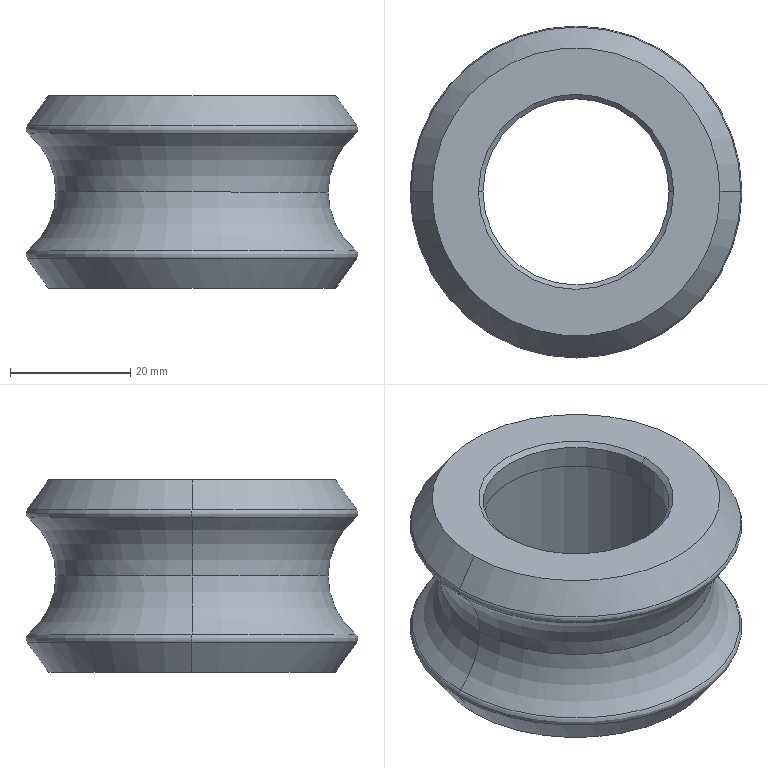Part | STEP file | ROLLER LINEAR GUIDE_01 | 1 solid | 31 faces | box 55.257 x 55.257 x 32 mm | volume 32346 mm3 | torus 10 | cylinder 8 | cone 8 | plane 5 | commonest cylinder face diameters 35 x4 31 x2 37.2 x2
STEP:
#1=CARTESIAN_POINT('',(-62.431,0.,-9.68));
#2=VERTEX_POINT('',#1);
#3=CARTESIAN_POINT('',(-57.839,0.,0.));
#4=VERTEX_POINT('',#3);
#5=CARTESIAN_POINT('',(-70.339,0.,0.));
#6=DIRECTION('',(0.,-1.,0.));
#7=DIRECTION('',(0.,0.,-1.));
#8=AXIS2_PLACEMENT_3D('',#5,#6,#7);
#9=CIRCLE('',#8,12.5);
#10=EDGE_CURVE('',#2,#4,#9,.T.);
#11=ORIENTED_EDGE('',*,*,#10,.T.);
#12=CARTESIAN_POINT('',(-12.5,0.,0.));
#13=VERTEX_POINT('',#12);
#14=CARTESIAN_POINT('',(-35.17,0.,0.));
#15=DIRECTION('',(0.,0.,-1.));
#16=DIRECTION('',(-1.,0.,0.));
#17=AXIS2_PLACEMENT_3D('',#14,#15,#16);
#18=CIRCLE('',#17,22.67);
#19=EDGE_CURVE('',#4,#13,#18,.T.);
#20=ORIENTED_EDGE('',*,*,#19,.T.);
#21=CARTESIAN_POINT('',(-7.908,0.,-9.68));
#22=VERTEX_POINT('',#21);
#23=CARTESIAN_POINT('',(0.,0.,0.));
#24=DIRECTION('',(0.,1.,0.));
#25=DIRECTION('',(-1.,0.,0.));
#26=AXIS2_PLACEMENT_3D('',#23,#24,#25);
#27=CIRCLE('',#26,12.5);
#28=EDGE_CURVE('',#22,#13,#27,.T.);
#29=ORIENTED_EDGE('',*,*,#28,.F.);
#30=CARTESIAN_POINT('',(-35.17,0.,-9.68));
#31=DIRECTION('',(0.,0.,1.));
#32=DIRECTION('',(1.,0.,0.));
#33=AXIS2_PLACEMENT_3D('',#30,#31,#32);
#34=CIRCLE('',#33,27.261);
#35=EDGE_CURVE('',#22,#2,#34,.T.);
#36=ORIENTED_EDGE('',*,*,#35,.T.);
#37=EDGE_LOOP('',(#11,#20,#29,#36));
#38=FACE_OUTER_BOUND('',#37,.T.);
#39=CARTESIAN_POINT('',(-35.17,0.,0.));
#40=DIRECTION('',(0.,0.,-1.));
#41=DIRECTION('',(-1.,0.,0.));
#42=AXIS2_PLACEMENT_3D('',#39,#40,#41);
#43=TOROIDAL_SURFACE('',#42,35.17,12.5);
#44=ADVANCED_FACE('',(#38),#43,.F.);
#45=ORIENTED_EDGE('',*,*,#28,.T.);
#46=CARTESIAN_POINT('',(-35.17,0.,0.));
#47=DIRECTION('',(0.,0.,-1.));
#48=DIRECTION('',(-1.,0.,0.));
#49=AXIS2_PLACEMENT_3D('',#46,#47,#48);
#50=CIRCLE('',#49,22.67);
#51=EDGE_CURVE('',#13,#4,#50,.T.);
#52=ORIENTED_EDGE('',*,*,#51,.T.);
#53=ORIENTED_EDGE('',*,*,#10,.F.);
#54=CARTESIAN_POINT('',(-35.17,0.,-9.68));
#55=DIRECTION('',(0.,0.,1.));
#56=DIRECTION('',(1.,0.,0.));
#57=AXIS2_PLACEMENT_3D('',#54,#55,#56);
#58=CIRCLE('',#57,27.261);
#59=EDGE_CURVE('',#2,#22,#58,.T.);
#60=ORIENTED_EDGE('',*,*,#59,.T.);
#61=EDGE_LOOP('',(#45,#52,#53,#60));
#62=FACE_OUTER_BOUND('',#61,.T.);
#63=CARTESIAN_POINT('',(-35.17,0.,0.));
#64=DIRECTION('',(0.,0.,-1.));
#65=DIRECTION('',(-1.,0.,0.));
#66=AXIS2_PLACEMENT_3D('',#63,#64,#65);
#67=TOROIDAL_SURFACE('',#66,35.17,12.5);
#68=ADVANCED_FACE('',(#62),#67,.F.);
#69=CARTESIAN_POINT('',(-16.57,0.,-11.8));
#70=VERTEX_POINT('',#69);
#71=CARTESIAN_POINT('',(-53.77,0.,-11.8));
#72=VERTEX_POINT('',#71);
#73=CARTESIAN_POINT('',(-35.17,0.,-11.8));
#74=DIRECTION('',(0.,0.,-1.));
#75=DIRECTION('',(-1.,0.,0.));
#76=AXIS2_PLACEMENT_3D('',#73,#74,#75);
#77=CIRCLE('',#76,18.6);
#78=EDGE_CURVE('',#70,#72,#77,.T.);
#79=ORIENTED_EDGE('',*,*,#78,.F.);
#80=CARTESIAN_POINT('',(-16.57,0.,-13.2));
#81=VERTEX_POINT('',#80);
#82=CARTESIAN_POINT('',(-16.57,0.,-16.));
#83=DIRECTION('',(0.,0.,-1.));
#84=VECTOR('',#83,1000.);
#85=LINE('',#82,#84);
#86=EDGE_CURVE('',#70,#81,#85,.T.);
#87=ORIENTED_EDGE('',*,*,#86,.T.);
#88=CARTESIAN_POINT('',(-53.77,0.,-13.2));
#89=VERTEX_POINT('',#88);
#90=CARTESIAN_POINT('',(-35.17,0.,-13.2));
#91=DIRECTION('',(0.,0.,-1.));
#92=DIRECTION('',(-1.,0.,0.));
#93=AXIS2_PLACEMENT_3D('',#90,#91,#92);
#94=CIRCLE('',#93,18.6);
#95=EDGE_CURVE('',#81,#89,#94,.T.);
#96=ORIENTED_EDGE('',*,*,#95,.T.);
#97=CARTESIAN_POINT('',(-53.77,0.,-16.));
#98=DIRECTION('',(0.,0.,-1.));
#99=VECTOR('',#98,1000.);
#100=LINE('',#97,#99);
#101=EDGE_CURVE('',#72,#89,#100,.T.);
#102=ORIENTED_EDGE('',*,*,#101,.F.);
#103=EDGE_LOOP('',(#79,#87,#96,#102));
#104=FACE_OUTER_BOUND('',#103,.T.);
#105=CARTESIAN_POINT('',(-35.17,0.,-16.));
#106=DIRECTION('',(0.,0.,-1.));
#107=DIRECTION('',(-1.,0.,0.));
#108=AXIS2_PLACEMENT_3D('',#105,#106,#107);
#109=CYLINDRICAL_SURFACE('',#108,18.6);
#110=ADVANCED_FACE('',(#104),#109,.F.);
#111=CARTESIAN_POINT('',(-62.431,0.,9.68));
#112=VERTEX_POINT('',#111);
#113=CARTESIAN_POINT('',(-7.908,0.,9.68));
#114=VERTEX_POINT('',#113);
#115=CARTESIAN_POINT('',(-35.17,0.,9.68));
#116=DIRECTION('',(0.,0.,-1.));
#117=DIRECTION('',(-1.,0.,0.));
#118=AXIS2_PLACEMENT_3D('',#115,#116,#117);
#119=CIRCLE('',#118,27.261);
#120=EDGE_CURVE('',#112,#114,#119,.T.);
#121=ORIENTED_EDGE('',*,*,#120,.F.);
#122=CARTESIAN_POINT('',(-62.617,0.,11.028));
#123=VERTEX_POINT('',#122);
#124=CARTESIAN_POINT('',(-61.798,0.,10.455));
#125=DIRECTION('',(0.,1.,0.));
#126=DIRECTION('',(-1.,0.,0.));
#127=AXIS2_PLACEMENT_3D('',#124,#125,#126);
#128=CIRCLE('',#127,1.);
#129=EDGE_CURVE('',#112,#123,#128,.T.);
#130=ORIENTED_EDGE('',*,*,#129,.T.);
#131=CARTESIAN_POINT('',(-7.722,0.,11.028));
#132=VERTEX_POINT('',#131);
#133=CARTESIAN_POINT('',(-35.17,0.,11.028));
#134=DIRECTION('',(0.,0.,1.));
#135=DIRECTION('',(1.,0.,0.));
#136=AXIS2_PLACEMENT_3D('',#133,#134,#135);
#137=CIRCLE('',#136,27.448);
#138=EDGE_CURVE('',#132,#123,#137,.T.);
#139=ORIENTED_EDGE('',*,*,#138,.F.);
#140=CARTESIAN_POINT('',(-8.541,0.,10.455));
#141=DIRECTION('',(0.,-1.,0.));
#142=DIRECTION('',(0.,0.,-1.));
#143=AXIS2_PLACEMENT_3D('',#140,#141,#142);
#144=CIRCLE('',#143,1.);
#145=EDGE_CURVE('',#114,#132,#144,.T.);
#146=ORIENTED_EDGE('',*,*,#145,.F.);
#147=EDGE_LOOP('',(#121,#130,#139,#146));
#148=FACE_OUTER_BOUND('',#147,.T.);
#149=CARTESIAN_POINT('',(-35.17,0.,10.455));
#150=DIRECTION('',(0.,0.,1.));
#151=DIRECTION('',(1.,0.,0.));
#152=AXIS2_PLACEMENT_3D('',#149,#150,#151);
#153=TOROIDAL_SURFACE('',#152,26.629,1.);
#154=ADVANCED_FACE('',(#148),#153,.T.);
#155=CARTESIAN_POINT('',(-62.617,0.,-11.028));
#156=VERTEX_POINT('',#155);
#157=CARTESIAN_POINT('',(-7.722,0.,-11.028));
#158=VERTEX_POINT('',#157);
#159=CARTESIAN_POINT('',(-35.17,0.,-11.028));
#160=DIRECTION('',(0.,0.,-1.));
#161=DIRECTION('',(-1.,0.,0.));
#162=AXIS2_PLACEMENT_3D('',#159,#160,#161);
#163=CIRCLE('',#162,27.448);
#164=EDGE_CURVE('',#156,#158,#163,.T.);
#165=ORIENTED_EDGE('',*,*,#164,.F.);
#166=CARTESIAN_POINT('',(-61.798,0.,-10.455));
#167=DIRECTION('',(0.,1.,0.));
#168=DIRECTION('',(-1.,0.,0.));
#169=AXIS2_PLACEMENT_3D('',#166,#167,#168);
#170=CIRCLE('',#169,1.);
#171=EDGE_CURVE('',#156,#2,#170,.T.);
#172=ORIENTED_EDGE('',*,*,#171,.T.);
#173=ORIENTED_EDGE('',*,*,#35,.F.);
#174=CARTESIAN_POINT('',(-8.541,0.,-10.455));
#175=DIRECTION('',(0.,-1.,0.));
#176=DIRECTION('',(0.,0.,-1.));
#177=AXIS2_PLACEMENT_3D('',#174,#175,#176);
#178=CIRCLE('',#177,1.);
#179=EDGE_CURVE('',#158,#22,#178,.T.);
#180=ORIENTED_EDGE('',*,*,#179,.F.);
#181=EDGE_LOOP('',(#165,#172,#173,#180));
#182=FACE_OUTER_BOUND('',#181,.T.);
#183=CARTESIAN_POINT('',(-35.17,0.,-10.455));
#184=DIRECTION('',(0.,0.,1.));
#185=DIRECTION('',(1.,0.,0.));
#186=AXIS2_PLACEMENT_3D('',#183,#184,#185);
#187=TOROIDAL_SURFACE('',#186,26.629,1.);
#188=ADVANCED_FACE('',(#182),#187,.T.);
#189=CARTESIAN_POINT('',(-17.67,0.,-15.25));
#190=VERTEX_POINT('',#189);
#191=CARTESIAN_POINT('',(-52.67,0.,-15.25));
#192=VERTEX_POINT('',#191);
#193=CARTESIAN_POINT('',(-35.17,0.,-15.25));
#194=DIRECTION('',(0.,0.,-1.));
#195=DIRECTION('',(1.,0.,0.));
#196=AXIS2_PLACEMENT_3D('',#193,#194,#195);
#197=CIRCLE('',#196,17.5);
#198=EDGE_CURVE('',#190,#192,#197,.T.);
#199=ORIENTED_EDGE('',*,*,#198,.F.);
#200=CARTESIAN_POINT('',(-16.92,0.,-16.));
#201=VERTEX_POINT('',#200);
#202=CARTESIAN_POINT('',(-17.67,0.,-15.25));
#203=DIRECTION('',(0.7071,0.,-0.7071));
#204=VECTOR('',#203,1000.);
#205=LINE('',#202,#204);
#206=EDGE_CURVE('',#190,#201,#205,.T.);
#207=ORIENTED_EDGE('',*,*,#206,.T.);
#208=CARTESIAN_POINT('',(-53.42,0.,-16.));
#209=VERTEX_POINT('',#208);
#210=CARTESIAN_POINT('',(-35.17,0.,-16.));
#211=DIRECTION('',(0.,0.,1.));
#212=DIRECTION('',(1.,0.,0.));
#213=AXIS2_PLACEMENT_3D('',#210,#211,#212);
#214=CIRCLE('',#213,18.25);
#215=EDGE_CURVE('',#209,#201,#214,.T.);
#216=ORIENTED_EDGE('',*,*,#215,.F.);
#217=CARTESIAN_POINT('',(-52.67,0.,-15.25));
#218=DIRECTION('',(-0.7071,0.,-0.7071));
#219=VECTOR('',#218,1000.);
#220=LINE('',#217,#219);
#221=EDGE_CURVE('',#192,#209,#220,.T.);
#222=ORIENTED_EDGE('',*,*,#221,.F.);
#223=EDGE_LOOP('',(#199,#207,#216,#222));
#224=FACE_OUTER_BOUND('',#223,.T.);
#225=CARTESIAN_POINT('',(-35.17,0.,-15.25));
#226=DIRECTION('',(0.,0.,-1.));
#227=DIRECTION('',(-1.,0.,0.));
#228=AXIS2_PLACEMENT_3D('',#225,#226,#227);
#229=CONICAL_SURFACE('',#228,17.5,0.7854);
#230=ADVANCED_FACE('',(#224),#229,.F.);
#231=CARTESIAN_POINT('',(-50.67,0.,15.25));
#232=VERTEX_POINT('',#231);
#233=CARTESIAN_POINT('',(-19.67,0.,15.25));
#234=VERTEX_POINT('',#233);
#235=CARTESIAN_POINT('',(-35.17,0.,15.25));
#236=DIRECTION('',(0.,0.,1.));
#237=DIRECTION('',(-1.,0.,0.));
#238=AXIS2_PLACEMENT_3D('',#235,#236,#237);
#239=CIRCLE('',#238,15.5);
#240=EDGE_CURVE('',#232,#234,#239,.T.);
#241=ORIENTED_EDGE('',*,*,#240,.F.);
#242=CARTESIAN_POINT('',(-51.42,0.,16.));
#243=VERTEX_POINT('',#242);
#244=CARTESIAN_POINT('',(-51.42,0.,16.));
#245=DIRECTION('',(-0.7071,0.,0.7071));
#246=VECTOR('',#245,1000.);
#247=LINE('',#244,#246);
#248=EDGE_CURVE('',#232,#243,#247,.T.);
#249=ORIENTED_EDGE('',*,*,#248,.T.);
#250=CARTESIAN_POINT('',(-18.92,0.,16.));
#251=VERTEX_POINT('',#250);
#252=CARTESIAN_POINT('',(-35.17,0.,16.));
#253=DIRECTION('',(0.,0.,-1.));
#254=DIRECTION('',(-1.,0.,0.));
#255=AXIS2_PLACEMENT_3D('',#252,#253,#254);
#256=CIRCLE('',#255,16.25);
#257=EDGE_CURVE('',#251,#243,#256,.T.);
#258=ORIENTED_EDGE('',*,*,#257,.F.);
#259=CARTESIAN_POINT('',(-18.92,0.,16.));
#260=DIRECTION('',(0.7071,0.,0.7071));
#261=VECTOR('',#260,1000.);
#262=LINE('',#259,#261);
#263=EDGE_CURVE('',#234,#251,#262,.T.);
#264=ORIENTED_EDGE('',*,*,#263,.F.);
#265=EDGE_LOOP('',(#241,#249,#258,#264));
#266=FACE_OUTER_BOUND('',#265,.T.);
#267=CARTESIAN_POINT('',(-35.17,0.,16.));
#268=DIRECTION('',(0.,0.,1.));
#269=DIRECTION('',(1.,0.,0.));
#270=AXIS2_PLACEMENT_3D('',#267,#268,#269);
#271=CONICAL_SURFACE('',#270,16.25,0.7854);
#272=ADVANCED_FACE('',(#266),#271,.F.);
#273=CARTESIAN_POINT('',(-17.87,0.,11.5));
#274=VERTEX_POINT('',#273);
#275=CARTESIAN_POINT('',(-52.47,0.,11.5));
#276=VERTEX_POINT('',#275);
#277=CARTESIAN_POINT('',(-35.17,0.,11.5));
#278=DIRECTION('',(0.,0.,-1.));
#279=DIRECTION('',(-1.,0.,0.));
#280=AXIS2_PLACEMENT_3D('',#277,#278,#279);
#281=CIRCLE('',#280,17.3);
#282=EDGE_CURVE('',#274,#276,#281,.T.);
#283=ORIENTED_EDGE('',*,*,#282,.F.);
#284=CARTESIAN_POINT('',(-17.67,0.,11.3));
#285=VERTEX_POINT('',#284);
#286=CARTESIAN_POINT('',(-17.87,0.,11.3));
#287=DIRECTION('',(0.,1.,0.));
#288=DIRECTION('',(-1.,0.,0.));
#289=AXIS2_PLACEMENT_3D('',#286,#287,#288);
#290=CIRCLE('',#289,0.2);
#291=EDGE_CURVE('',#274,#285,#290,.T.);
#292=ORIENTED_EDGE('',*,*,#291,.T.);
#293=CARTESIAN_POINT('',(-52.67,0.,11.3));
#294=VERTEX_POINT('',#293);
#295=CARTESIAN_POINT('',(-35.17,0.,11.3));
#296=DIRECTION('',(0.,0.,1.));
#297=DIRECTION('',(-1.,0.,0.));
#298=AXIS2_PLACEMENT_3D('',#295,#296,#297);
#299=CIRCLE('',#298,17.5);
#300=EDGE_CURVE('',#294,#285,#299,.T.);
#301=ORIENTED_EDGE('',*,*,#300,.F.);
#302=CARTESIAN_POINT('',(-52.47,0.,11.3));
#303=DIRECTION('',(0.,-1.,0.));
#304=DIRECTION('',(0.,0.,-1.));
#305=AXIS2_PLACEMENT_3D('',#302,#303,#304);
#306=CIRCLE('',#305,0.2);
#307=EDGE_CURVE('',#276,#294,#306,.T.);
#308=ORIENTED_EDGE('',*,*,#307,.F.);
#309=EDGE_LOOP('',(#283,#292,#301,#308));
#310=FACE_OUTER_BOUND('',#309,.T.);
#311=CARTESIAN_POINT('',(-35.17,0.,11.3));
#312=DIRECTION('',(0.,0.,-1.));
#313=DIRECTION('',(-1.,0.,0.));
#314=AXIS2_PLACEMENT_3D('',#311,#312,#313);
#315=TOROIDAL_SURFACE('',#314,17.3,0.2);
#316=ADVANCED_FACE('',(#310),#315,.F.);
#317=ORIENTED_EDGE('',*,*,#240,.T.);
#318=CARTESIAN_POINT('',(-19.67,0.,11.5));
#319=VERTEX_POINT('',#318);
#320=CARTESIAN_POINT('',(-19.67,0.,31.5));
#321=DIRECTION('',(0.,0.,-1.));
#322=VECTOR('',#321,1000.);
#323=LINE('',#320,#322);
#324=EDGE_CURVE('',#234,#319,#323,.T.);
#325=ORIENTED_EDGE('',*,*,#324,.T.);
#326=CARTESIAN_POINT('',(-50.67,0.,11.5));
#327=VERTEX_POINT('',#326);
#328=CARTESIAN_POINT('',(-35.17,0.,11.5));
#329=DIRECTION('',(0.,0.,-1.));
#330=DIRECTION('',(-1.,0.,0.));
#331=AXIS2_PLACEMENT_3D('',#328,#329,#330);
#332=CIRCLE('',#331,15.5);
#333=EDGE_CURVE('',#319,#327,#332,.T.);
#334=ORIENTED_EDGE('',*,*,#333,.T.);
#335=CARTESIAN_POINT('',(-50.67,0.,31.5));
#336=DIRECTION('',(0.,0.,-1.));
#337=VECTOR('',#336,1000.);
#338=LINE('',#335,#337);
#339=EDGE_CURVE('',#232,#327,#338,.T.);
#340=ORIENTED_EDGE('',*,*,#339,.F.);
#341=EDGE_LOOP('',(#317,#325,#334,#340));
#342=FACE_OUTER_BOUND('',#341,.T.);
#343=CARTESIAN_POINT('',(-35.17,0.,31.5));
#344=DIRECTION('',(0.,0.,-1.));
#345=DIRECTION('',(-1.,0.,0.));
#346=AXIS2_PLACEMENT_3D('',#343,#344,#345);
#347=CYLINDRICAL_SURFACE('',#346,15.5);
#348=ADVANCED_FACE('',(#342),#347,.F.);
#349=CARTESIAN_POINT('',(-52.67,0.,-13.2));
#350=VERTEX_POINT('',#349);
#351=CARTESIAN_POINT('',(-17.67,0.,-13.2));
#352=VERTEX_POINT('',#351);
#353=CARTESIAN_POINT('',(-35.17,0.,-13.2));
#354=DIRECTION('',(0.,0.,1.));
#355=DIRECTION('',(-1.,0.,0.));
#356=AXIS2_PLACEMENT_3D('',#353,#354,#355);
#357=CIRCLE('',#356,17.5);
#358=EDGE_CURVE('',#350,#352,#357,.T.);
#359=ORIENTED_EDGE('',*,*,#358,.T.);
#360=CARTESIAN_POINT('',(-17.67,0.,11.5));
#361=DIRECTION('',(0.,0.,-1.));
#362=VECTOR('',#361,1000.);
#363=LINE('',#360,#362);
#364=EDGE_CURVE('',#352,#190,#363,.T.);
#365=ORIENTED_EDGE('',*,*,#364,.T.);
#366=ORIENTED_EDGE('',*,*,#198,.T.);
#367=CARTESIAN_POINT('',(-52.67,0.,11.5));
#368=DIRECTION('',(0.,0.,-1.));
#369=VECTOR('',#368,1000.);
#370=LINE('',#367,#369);
#371=EDGE_CURVE('',#350,#192,#370,.T.);
#372=ORIENTED_EDGE('',*,*,#371,.F.);
#373=EDGE_LOOP('',(#359,#365,#366,#372));
#374=FACE_OUTER_BOUND('',#373,.T.);
#375=CARTESIAN_POINT('',(-35.17,0.,11.5));
#376=DIRECTION('',(0.,0.,-1.));
#377=DIRECTION('',(-1.,0.,0.));
#378=AXIS2_PLACEMENT_3D('',#375,#376,#377);
#379=CYLINDRICAL_SURFACE('',#378,17.5);
#380=ADVANCED_FACE('',(#374),#379,.F.);
#381=CARTESIAN_POINT('',(-59.136,0.,-16.));
#382=VERTEX_POINT('',#381);
#383=CARTESIAN_POINT('',(-11.203,0.,-16.));
#384=VERTEX_POINT('',#383);
#385=CARTESIAN_POINT('',(-35.17,0.,-16.));
#386=DIRECTION('',(0.,0.,-1.));
#387=DIRECTION('',(-1.,0.,0.));
#388=AXIS2_PLACEMENT_3D('',#385,#386,#387);
#389=CIRCLE('',#388,23.966);
#390=EDGE_CURVE('',#382,#384,#389,.T.);
#391=ORIENTED_EDGE('',*,*,#390,.F.);
#392=CARTESIAN_POINT('',(-63.17,0.,-10.239));
#393=DIRECTION('',(-0.5736,0.,0.8192));
#394=VECTOR('',#393,1000.);
#395=LINE('',#392,#394);
#396=EDGE_CURVE('',#382,#156,#395,.T.);
#397=ORIENTED_EDGE('',*,*,#396,.T.);
#398=ORIENTED_EDGE('',*,*,#164,.T.);
#399=CARTESIAN_POINT('',(-7.17,0.,-10.239));
#400=DIRECTION('',(0.5736,0.,0.8192));
#401=VECTOR('',#400,1000.);
#402=LINE('',#399,#401);
#403=EDGE_CURVE('',#384,#158,#402,.T.);
#404=ORIENTED_EDGE('',*,*,#403,.F.);
#405=EDGE_LOOP('',(#391,#397,#398,#404));
#406=FACE_OUTER_BOUND('',#405,.T.);
#407=CARTESIAN_POINT('',(-35.17,0.,-10.239));
#408=DIRECTION('',(0.,0.,1.));
#409=DIRECTION('',(1.,0.,0.));
#410=AXIS2_PLACEMENT_3D('',#407,#408,#409);
#411=CONICAL_SURFACE('',#410,28.,0.6109);
#412=ADVANCED_FACE('',(#406),#411,.T.);
#413=CARTESIAN_POINT('',(-59.136,0.,16.));
#414=VERTEX_POINT('',#413);
#415=CARTESIAN_POINT('',(-11.203,0.,16.));
#416=VERTEX_POINT('',#415);
#417=CARTESIAN_POINT('',(-35.17,0.,16.));
#418=DIRECTION('',(0.,0.,-1.));
#419=DIRECTION('',(-1.,0.,0.));
#420=AXIS2_PLACEMENT_3D('',#417,#418,#419);
#421=CIRCLE('',#420,23.966);
#422=EDGE_CURVE('',#414,#416,#421,.T.);
#423=ORIENTED_EDGE('',*,*,#422,.T.);
#424=CARTESIAN_POINT('',(-11.203,0.,16.));
#425=DIRECTION('',(0.5736,0.,-0.8192));
#426=VECTOR('',#425,1000.);
#427=LINE('',#424,#426);
#428=EDGE_CURVE('',#416,#132,#427,.T.);
#429=ORIENTED_EDGE('',*,*,#428,.T.);
#430=ORIENTED_EDGE('',*,*,#138,.T.);
#431=CARTESIAN_POINT('',(-59.136,0.,16.));
#432=DIRECTION('',(-0.5736,0.,-0.8192));
#433=VECTOR('',#432,1000.);
#434=LINE('',#431,#433);
#435=EDGE_CURVE('',#414,#123,#434,.T.);
#436=ORIENTED_EDGE('',*,*,#435,.F.);
#437=EDGE_LOOP('',(#423,#429,#430,#436));
#438=FACE_OUTER_BOUND('',#437,.T.);
#439=CARTESIAN_POINT('',(-35.17,0.,16.));
#440=DIRECTION('',(0.,0.,-1.));
#441=DIRECTION('',(-1.,0.,0.));
#442=AXIS2_PLACEMENT_3D('',#439,#440,#441);
#443=CONICAL_SURFACE('',#442,23.966,0.6109);
#444=ADVANCED_FACE('',(#438),#443,.T.);
#445=ORIENTED_EDGE('',*,*,#51,.F.);
#446=CARTESIAN_POINT('',(0.,0.,0.));
#447=DIRECTION('',(0.,1.,0.));
#448=DIRECTION('',(-1.,0.,0.));
#449=AXIS2_PLACEMENT_3D('',#446,#447,#448);
#450=CIRCLE('',#449,12.5);
#451=EDGE_CURVE('',#13,#114,#450,.T.);
#452=ORIENTED_EDGE('',*,*,#451,.T.);
#453=CARTESIAN_POINT('',(-35.17,0.,9.68));
#454=DIRECTION('',(0.,0.,-1.));
#455=DIRECTION('',(-1.,0.,0.));
#456=AXIS2_PLACEMENT_3D('',#453,#454,#455);
#457=CIRCLE('',#456,27.261);
#458=EDGE_CURVE('',#114,#112,#457,.T.);
#459=ORIENTED_EDGE('',*,*,#458,.T.);
#460=CARTESIAN_POINT('',(-70.339,0.,0.));
#461=DIRECTION('',(0.,-1.,0.));
#462=DIRECTION('',(0.,0.,-1.));
#463=AXIS2_PLACEMENT_3D('',#460,#461,#462);
#464=CIRCLE('',#463,12.5);
#465=EDGE_CURVE('',#4,#112,#464,.T.);
#466=ORIENTED_EDGE('',*,*,#465,.F.);
#467=EDGE_LOOP('',(#445,#452,#459,#466));
#468=FACE_OUTER_BOUND('',#467,.T.);
#469=CARTESIAN_POINT('',(-35.17,0.,0.));
#470=DIRECTION('',(0.,0.,-1.));
#471=DIRECTION('',(-1.,0.,0.));
#472=AXIS2_PLACEMENT_3D('',#469,#470,#471);
#473=TOROIDAL_SURFACE('',#472,35.17,12.5);
#474=ADVANCED_FACE('',(#468),#473,.F.);
#475=ORIENTED_EDGE('',*,*,#300,.T.);
#476=CARTESIAN_POINT('',(-17.67,0.,-11.8));
#477=VERTEX_POINT('',#476);
#478=CARTESIAN_POINT('',(-17.67,0.,11.5));
#479=DIRECTION('',(0.,0.,-1.));
#480=VECTOR('',#479,1000.);
#481=LINE('',#478,#480);
#482=EDGE_CURVE('',#285,#477,#481,.T.);
#483=ORIENTED_EDGE('',*,*,#482,.T.);
#484=CARTESIAN_POINT('',(-52.67,0.,-11.8));
#485=VERTEX_POINT('',#484);
#486=CARTESIAN_POINT('',(-35.17,0.,-11.8));
#487=DIRECTION('',(0.,0.,-1.));
#488=DIRECTION('',(1.,0.,0.));
#489=AXIS2_PLACEMENT_3D('',#486,#487,#488);
#490=CIRCLE('',#489,17.5);
#491=EDGE_CURVE('',#477,#485,#490,.T.);
#492=ORIENTED_EDGE('',*,*,#491,.T.);
#493=CARTESIAN_POINT('',(-52.67,0.,11.5));
#494=DIRECTION('',(0.,0.,-1.));
#495=VECTOR('',#494,1000.);
#496=LINE('',#493,#495);
#497=EDGE_CURVE('',#294,#485,#496,.T.);
#498=ORIENTED_EDGE('',*,*,#497,.F.);
#499=EDGE_LOOP('',(#475,#483,#492,#498));
#500=FACE_OUTER_BOUND('',#499,.T.);
#501=CARTESIAN_POINT('',(-35.17,0.,11.5));
#502=DIRECTION('',(0.,0.,-1.));
#503=DIRECTION('',(-1.,0.,0.));
#504=AXIS2_PLACEMENT_3D('',#501,#502,#503);
#505=CYLINDRICAL_SURFACE('',#504,17.5);
#506=ADVANCED_FACE('',(#500),#505,.F.);
#507=ORIENTED_EDGE('',*,*,#482,.F.);
#508=CARTESIAN_POINT('',(-35.17,0.,11.3));
#509=DIRECTION('',(0.,0.,1.));
#510=DIRECTION('',(-1.,0.,0.));
#511=AXIS2_PLACEMENT_3D('',#508,#509,#510);
#512=CIRCLE('',#511,17.5);
#513=EDGE_CURVE('',#285,#294,#512,.T.);
#514=ORIENTED_EDGE('',*,*,#513,.T.);
#515=ORIENTED_EDGE('',*,*,#497,.T.);
#516=CARTESIAN_POINT('',(-35.17,0.,-11.8));
#517=DIRECTION('',(0.,0.,-1.));
#518=DIRECTION('',(1.,0.,0.));
#519=AXIS2_PLACEMENT_3D('',#516,#517,#518);
#520=CIRCLE('',#519,17.5);
#521=EDGE_CURVE('',#485,#477,#520,.T.);
#522=ORIENTED_EDGE('',*,*,#521,.T.);
#523=EDGE_LOOP('',(#507,#514,#515,#522));
#524=FACE_OUTER_BOUND('',#523,.T.);
#525=CARTESIAN_POINT('',(-35.17,0.,11.5));
#526=DIRECTION('',(0.,0.,-1.));
#527=DIRECTION('',(-1.,0.,0.));
#528=AXIS2_PLACEMENT_3D('',#525,#526,#527);
#529=CYLINDRICAL_SURFACE('',#528,17.5);
#530=ADVANCED_FACE('',(#524),#529,.F.);
#531=ORIENTED_EDGE('',*,*,#19,.F.);
#532=ORIENTED_EDGE('',*,*,#465,.T.);
#533=ORIENTED_EDGE('',*,*,#120,.T.);
#534=ORIENTED_EDGE('',*,*,#451,.F.);
#535=EDGE_LOOP('',(#531,#532,#533,#534));
#536=FACE_OUTER_BOUND('',#535,.T.);
#537=CARTESIAN_POINT('',(-35.17,0.,0.));
#538=DIRECTION('',(0.,0.,-1.));
#539=DIRECTION('',(-1.,0.,0.));
#540=AXIS2_PLACEMENT_3D('',#537,#538,#539);
#541=TOROIDAL_SURFACE('',#540,35.17,12.5);
#542=ADVANCED_FACE('',(#536),#541,.F.);
#543=ORIENTED_EDGE('',*,*,#428,.F.);
#544=CARTESIAN_POINT('',(-35.17,0.,16.));
#545=DIRECTION('',(0.,0.,-1.));
#546=DIRECTION('',(-1.,0.,0.));
#547=AXIS2_PLACEMENT_3D('',#544,#545,#546);
#548=CIRCLE('',#547,23.966);
#549=EDGE_CURVE('',#416,#414,#548,.T.);
#550=ORIENTED_EDGE('',*,*,#549,.T.);
#551=ORIENTED_EDGE('',*,*,#435,.T.);
#552=CARTESIAN_POINT('',(-35.17,0.,11.028));
#553=DIRECTION('',(0.,0.,1.));
#554=DIRECTION('',(1.,0.,0.));
#555=AXIS2_PLACEMENT_3D('',#552,#553,#554);
#556=CIRCLE('',#555,27.448);
#557=EDGE_CURVE('',#123,#132,#556,.T.);
#558=ORIENTED_EDGE('',*,*,#557,.T.);
#559=EDGE_LOOP('',(#543,#550,#551,#558));
#560=FACE_OUTER_BOUND('',#559,.T.);
#561=CARTESIAN_POINT('',(-35.17,0.,16.));
#562=DIRECTION('',(0.,0.,-1.));
#563=DIRECTION('',(-1.,0.,0.));
#564=AXIS2_PLACEMENT_3D('',#561,#562,#563);
#565=CONICAL_SURFACE('',#564,23.966,0.6109);
#566=ADVANCED_FACE('',(#560),#565,.T.);
#567=ORIENTED_EDGE('',*,*,#257,.T.);
#568=CARTESIAN_POINT('',(-35.17,0.,16.));
#569=DIRECTION('',(0.,0.,-1.));
#570=DIRECTION('',(-1.,0.,0.));
#571=AXIS2_PLACEMENT_3D('',#568,#569,#570);
#572=CIRCLE('',#571,16.25);
#573=EDGE_CURVE('',#243,#251,#572,.T.);
#574=ORIENTED_EDGE('',*,*,#573,.T.);
#575=EDGE_LOOP('',(#567,#574));
#576=FACE_BOUND('',#575,.T.);
#577=ORIENTED_EDGE('',*,*,#422,.F.);
#578=ORIENTED_EDGE('',*,*,#549,.F.);
#579=EDGE_LOOP('',(#577,#578));
#580=FACE_OUTER_BOUND('',#579,.T.);
#581=CARTESIAN_POINT('',(-11.203,0.,16.));
#582=DIRECTION('',(0.,0.,-1.));
#583=DIRECTION('',(-1.,0.,0.));
#584=AXIS2_PLACEMENT_3D('',#581,#582,#583);
#585=PLANE('',#584);
#586=ADVANCED_FACE('',(#576,#580),#585,.F.);
#587=ORIENTED_EDGE('',*,*,#215,.T.);
#588=CARTESIAN_POINT('',(-35.17,0.,-16.));
#589=DIRECTION('',(0.,0.,1.));
#590=DIRECTION('',(1.,0.,0.));
#591=AXIS2_PLACEMENT_3D('',#588,#589,#590);
#592=CIRCLE('',#591,18.25);
#593=EDGE_CURVE('',#201,#209,#592,.T.);
#594=ORIENTED_EDGE('',*,*,#593,.T.);
#595=EDGE_LOOP('',(#587,#594));
#596=FACE_BOUND('',#595,.T.);
#597=CARTESIAN_POINT('',(-35.17,0.,-16.));
#598=DIRECTION('',(0.,0.,-1.));
#599=DIRECTION('',(-1.,0.,0.));
#600=AXIS2_PLACEMENT_3D('',#597,#598,#599);
#601=CIRCLE('',#600,23.966);
#602=EDGE_CURVE('',#384,#382,#601,.T.);
#603=ORIENTED_EDGE('',*,*,#602,.T.);
#604=ORIENTED_EDGE('',*,*,#390,.T.);
#605=EDGE_LOOP('',(#603,#604));
#606=FACE_OUTER_BOUND('',#605,.T.);
#607=CARTESIAN_POINT('',(-11.203,0.,-16.));
#608=DIRECTION('',(0.,0.,1.));
#609=DIRECTION('',(1.,0.,0.));
#610=AXIS2_PLACEMENT_3D('',#607,#608,#609);
#611=PLANE('',#610);
#612=ADVANCED_FACE('',(#596,#606),#611,.F.);
#613=ORIENTED_EDGE('',*,*,#396,.F.);
#614=ORIENTED_EDGE('',*,*,#602,.F.);
#615=ORIENTED_EDGE('',*,*,#403,.T.);
#616=CARTESIAN_POINT('',(-35.17,0.,-11.028));
#617=DIRECTION('',(0.,0.,-1.));
#618=DIRECTION('',(-1.,0.,0.));
#619=AXIS2_PLACEMENT_3D('',#616,#617,#618);
#620=CIRCLE('',#619,27.448);
#621=EDGE_CURVE('',#158,#156,#620,.T.);
#622=ORIENTED_EDGE('',*,*,#621,.T.);
#623=EDGE_LOOP('',(#613,#614,#615,#622));
#624=FACE_OUTER_BOUND('',#623,.T.);
#625=CARTESIAN_POINT('',(-35.17,0.,-10.239));
#626=DIRECTION('',(0.,0.,1.));
#627=DIRECTION('',(1.,0.,0.));
#628=AXIS2_PLACEMENT_3D('',#625,#626,#627);
#629=CONICAL_SURFACE('',#628,28.,0.6109);
#630=ADVANCED_FACE('',(#624),#629,.T.);
#631=ORIENTED_EDGE('',*,*,#364,.F.);
#632=CARTESIAN_POINT('',(-35.17,0.,-13.2));
#633=DIRECTION('',(0.,0.,1.));
#634=DIRECTION('',(-1.,0.,0.));
#635=AXIS2_PLACEMENT_3D('',#632,#633,#634);
#636=CIRCLE('',#635,17.5);
#637=EDGE_CURVE('',#352,#350,#636,.T.);
#638=ORIENTED_EDGE('',*,*,#637,.T.);
#639=ORIENTED_EDGE('',*,*,#371,.T.);
#640=CARTESIAN_POINT('',(-35.17,0.,-15.25));
#641=DIRECTION('',(0.,0.,-1.));
#642=DIRECTION('',(1.,0.,0.));
#643=AXIS2_PLACEMENT_3D('',#640,#641,#642);
#644=CIRCLE('',#643,17.5);
#645=EDGE_CURVE('',#192,#190,#644,.T.);
#646=ORIENTED_EDGE('',*,*,#645,.T.);
#647=EDGE_LOOP('',(#631,#638,#639,#646));
#648=FACE_OUTER_BOUND('',#647,.T.);
#649=CARTESIAN_POINT('',(-35.17,0.,11.5));
#650=DIRECTION('',(0.,0.,-1.));
#651=DIRECTION('',(-1.,0.,0.));
#652=AXIS2_PLACEMENT_3D('',#649,#650,#651);
#653=CYLINDRICAL_SURFACE('',#652,17.5);
#654=ADVANCED_FACE('',(#648),#653,.F.);
#655=CARTESIAN_POINT('',(-35.17,0.,11.5));
#656=DIRECTION('',(0.,0.,-1.));
#657=DIRECTION('',(-1.,0.,0.));
#658=AXIS2_PLACEMENT_3D('',#655,#656,#657);
#659=CIRCLE('',#658,17.3);
#660=EDGE_CURVE('',#276,#274,#659,.T.);
#661=ORIENTED_EDGE('',*,*,#660,.T.);
#662=ORIENTED_EDGE('',*,*,#282,.T.);
#663=EDGE_LOOP('',(#661,#662));
#664=FACE_OUTER_BOUND('',#663,.T.);
#665=CARTESIAN_POINT('',(-35.17,0.,11.5));
#666=DIRECTION('',(0.,0.,-1.));
#667=DIRECTION('',(-1.,0.,0.));
#668=AXIS2_PLACEMENT_3D('',#665,#666,#667);
#669=CIRCLE('',#668,15.5);
#670=EDGE_CURVE('',#327,#319,#669,.T.);
#671=ORIENTED_EDGE('',*,*,#670,.F.);
#672=ORIENTED_EDGE('',*,*,#333,.F.);
#673=EDGE_LOOP('',(#671,#672));
#674=FACE_BOUND('',#673,.T.);
#675=CARTESIAN_POINT('',(-35.17,0.,11.5));
#676=DIRECTION('',(0.,0.,-1.));
#677=DIRECTION('',(-1.,0.,0.));
#678=AXIS2_PLACEMENT_3D('',#675,#676,#677);
#679=PLANE('',#678);
#680=ADVANCED_FACE('',(#664,#674),#679,.T.);
#681=ORIENTED_EDGE('',*,*,#324,.F.);
#682=CARTESIAN_POINT('',(-35.17,0.,15.25));
#683=DIRECTION('',(0.,0.,1.));
#684=DIRECTION('',(-1.,0.,0.));
#685=AXIS2_PLACEMENT_3D('',#682,#683,#684);
#686=CIRCLE('',#685,15.5);
#687=EDGE_CURVE('',#234,#232,#686,.T.);
#688=ORIENTED_EDGE('',*,*,#687,.T.);
#689=ORIENTED_EDGE('',*,*,#339,.T.);
#690=ORIENTED_EDGE('',*,*,#670,.T.);
#691=EDGE_LOOP('',(#681,#688,#689,#690));
#692=FACE_OUTER_BOUND('',#691,.T.);
#693=CARTESIAN_POINT('',(-35.17,0.,31.5));
#694=DIRECTION('',(0.,0.,-1.));
#695=DIRECTION('',(-1.,0.,0.));
#696=AXIS2_PLACEMENT_3D('',#693,#694,#695);
#697=CYLINDRICAL_SURFACE('',#696,15.5);
#698=ADVANCED_FACE('',(#692),#697,.F.);
#699=ORIENTED_EDGE('',*,*,#291,.F.);
#700=ORIENTED_EDGE('',*,*,#660,.F.);
#701=ORIENTED_EDGE('',*,*,#307,.T.);
#702=ORIENTED_EDGE('',*,*,#513,.F.);
#703=EDGE_LOOP('',(#699,#700,#701,#702));
#704=FACE_OUTER_BOUND('',#703,.T.);
#705=CARTESIAN_POINT('',(-35.17,0.,11.3));
#706=DIRECTION('',(0.,0.,-1.));
#707=DIRECTION('',(-1.,0.,0.));
#708=AXIS2_PLACEMENT_3D('',#705,#706,#707);
#709=TOROIDAL_SURFACE('',#708,17.3,0.2);
#710=ADVANCED_FACE('',(#704),#709,.F.);
#711=ORIENTED_EDGE('',*,*,#248,.F.);
#712=ORIENTED_EDGE('',*,*,#687,.F.);
#713=ORIENTED_EDGE('',*,*,#263,.T.);
#714=ORIENTED_EDGE('',*,*,#573,.F.);
#715=EDGE_LOOP('',(#711,#712,#713,#714));
#716=FACE_OUTER_BOUND('',#715,.T.);
#717=CARTESIAN_POINT('',(-35.17,0.,16.));
#718=DIRECTION('',(0.,0.,1.));
#719=DIRECTION('',(1.,0.,0.));
#720=AXIS2_PLACEMENT_3D('',#717,#718,#719);
#721=CONICAL_SURFACE('',#720,16.25,0.7854);
#722=ADVANCED_FACE('',(#716),#721,.F.);
#723=ORIENTED_EDGE('',*,*,#206,.F.);
#724=ORIENTED_EDGE('',*,*,#645,.F.);
#725=ORIENTED_EDGE('',*,*,#221,.T.);
#726=ORIENTED_EDGE('',*,*,#593,.F.);
#727=EDGE_LOOP('',(#723,#724,#725,#726));
#728=FACE_OUTER_BOUND('',#727,.T.);
#729=CARTESIAN_POINT('',(-35.17,0.,-15.25));
#730=DIRECTION('',(0.,0.,-1.));
#731=DIRECTION('',(-1.,0.,0.));
#732=AXIS2_PLACEMENT_3D('',#729,#730,#731);
#733=CONICAL_SURFACE('',#732,17.5,0.7854);
#734=ADVANCED_FACE('',(#728),#733,.F.);
#735=ORIENTED_EDGE('',*,*,#171,.F.);
#736=ORIENTED_EDGE('',*,*,#621,.F.);
#737=ORIENTED_EDGE('',*,*,#179,.T.);
#738=ORIENTED_EDGE('',*,*,#59,.F.);
#739=EDGE_LOOP('',(#735,#736,#737,#738));
#740=FACE_OUTER_BOUND('',#739,.T.);
#741=CARTESIAN_POINT('',(-35.17,0.,-10.455));
#742=DIRECTION('',(0.,0.,1.));
#743=DIRECTION('',(1.,0.,0.));
#744=AXIS2_PLACEMENT_3D('',#741,#742,#743);
#745=TOROIDAL_SURFACE('',#744,26.629,1.);
#746=ADVANCED_FACE('',(#740),#745,.T.);
#747=ORIENTED_EDGE('',*,*,#129,.F.);
#748=ORIENTED_EDGE('',*,*,#458,.F.);
#749=ORIENTED_EDGE('',*,*,#145,.T.);
#750=ORIENTED_EDGE('',*,*,#557,.F.);
#751=EDGE_LOOP('',(#747,#748,#749,#750));
#752=FACE_OUTER_BOUND('',#751,.T.);
#753=CARTESIAN_POINT('',(-35.17,0.,10.455));
#754=DIRECTION('',(0.,0.,1.));
#755=DIRECTION('',(1.,0.,0.));
#756=AXIS2_PLACEMENT_3D('',#753,#754,#755);
#757=TOROIDAL_SURFACE('',#756,26.629,1.);
#758=ADVANCED_FACE('',(#752),#757,.T.);
#759=CARTESIAN_POINT('',(-35.17,0.,-11.8));
#760=DIRECTION('',(0.,0.,-1.));
#761=DIRECTION('',(-1.,0.,0.));
#762=AXIS2_PLACEMENT_3D('',#759,#760,#761);
#763=CIRCLE('',#762,18.6);
#764=EDGE_CURVE('',#72,#70,#763,.T.);
#765=ORIENTED_EDGE('',*,*,#764,.T.);
#766=ORIENTED_EDGE('',*,*,#78,.T.);
#767=EDGE_LOOP('',(#765,#766));
#768=FACE_OUTER_BOUND('',#767,.T.);
#769=ORIENTED_EDGE('',*,*,#521,.F.);
#770=ORIENTED_EDGE('',*,*,#491,.F.);
#771=EDGE_LOOP('',(#769,#770));
#772=FACE_BOUND('',#771,.T.);
#773=CARTESIAN_POINT('',(-51.217,0.,-11.8));
#774=DIRECTION('',(0.,0.,1.));
#775=DIRECTION('',(1.,0.,0.));
#776=AXIS2_PLACEMENT_3D('',#773,#774,#775);
#777=PLANE('',#776);
#778=ADVANCED_FACE('',(#768,#772),#777,.F.);
#779=CARTESIAN_POINT('',(-35.17,0.,-13.2));
#780=DIRECTION('',(0.,0.,-1.));
#781=DIRECTION('',(-1.,0.,0.));
#782=AXIS2_PLACEMENT_3D('',#779,#780,#781);
#783=CIRCLE('',#782,18.6);
#784=EDGE_CURVE('',#89,#81,#783,.T.);
#785=ORIENTED_EDGE('',*,*,#784,.F.);
#786=ORIENTED_EDGE('',*,*,#95,.F.);
#787=EDGE_LOOP('',(#785,#786));
#788=FACE_OUTER_BOUND('',#787,.T.);
#789=ORIENTED_EDGE('',*,*,#358,.F.);
#790=ORIENTED_EDGE('',*,*,#637,.F.);
#791=EDGE_LOOP('',(#789,#790));
#792=FACE_BOUND('',#791,.T.);
#793=CARTESIAN_POINT('',(-51.217,0.,-13.2));
#794=DIRECTION('',(0.,0.,-1.));
#795=DIRECTION('',(-1.,0.,0.));
#796=AXIS2_PLACEMENT_3D('',#793,#794,#795);
#797=PLANE('',#796);
#798=ADVANCED_FACE('',(#788,#792),#797,.F.);
#799=ORIENTED_EDGE('',*,*,#86,.F.);
#800=ORIENTED_EDGE('',*,*,#764,.F.);
#801=ORIENTED_EDGE('',*,*,#101,.T.);
#802=ORIENTED_EDGE('',*,*,#784,.T.);
#803=EDGE_LOOP('',(#799,#800,#801,#802));
#804=FACE_OUTER_BOUND('',#803,.T.);
#805=CARTESIAN_POINT('',(-35.17,0.,-16.));
#806=DIRECTION('',(0.,0.,-1.));
#807=DIRECTION('',(-1.,0.,0.));
#808=AXIS2_PLACEMENT_3D('',#805,#806,#807);
#809=CYLINDRICAL_SURFACE('',#808,18.6);
#810=ADVANCED_FACE('',(#804),#809,.F.);
#811=CLOSED_SHELL('',(#44,#68,#110,#154,#188,#230,#272,#316,#348,#380,#412,#444,#474,#506,#530,#542,#566,#586,#612,#630,#654,#680,#698,#710,#722,#734,#746,#758,#778,#798,#810));
#812=MANIFOLD_SOLID_BREP('',#811);
#813=CARTESIAN_POINT('',(0.,0.,0.));
#814=DIRECTION('',(0.,0.,1.));
#815=DIRECTION('',(1.,0.,0.));
#816=AXIS2_PLACEMENT_3D('',#813,#814,#815);
#817=(LENGTH_UNIT()NAMED_UNIT(*)SI_UNIT(.MILLI.,.METRE.));
#818=UNCERTAINTY_MEASURE_WITH_UNIT(LENGTH_MEASURE(0.00001),#817,'','');
#819=(NAMED_UNIT(*)PLANE_ANGLE_UNIT()SI_UNIT($,.RADIAN.));
#820=(NAMED_UNIT(*)SI_UNIT($,.STERADIAN.)SOLID_ANGLE_UNIT());
#821=(GEOMETRIC_REPRESENTATION_CONTEXT(3)GLOBAL_UNCERTAINTY_ASSIGNED_CONTEXT((#818))GLOBAL_UNIT_ASSIGNED_CONTEXT((#817,#819,#820))REPRESENTATION_CONTEXT('',''));
#822=ADVANCED_BREP_SHAPE_REPRESENTATION('',(#812,#816),#821);